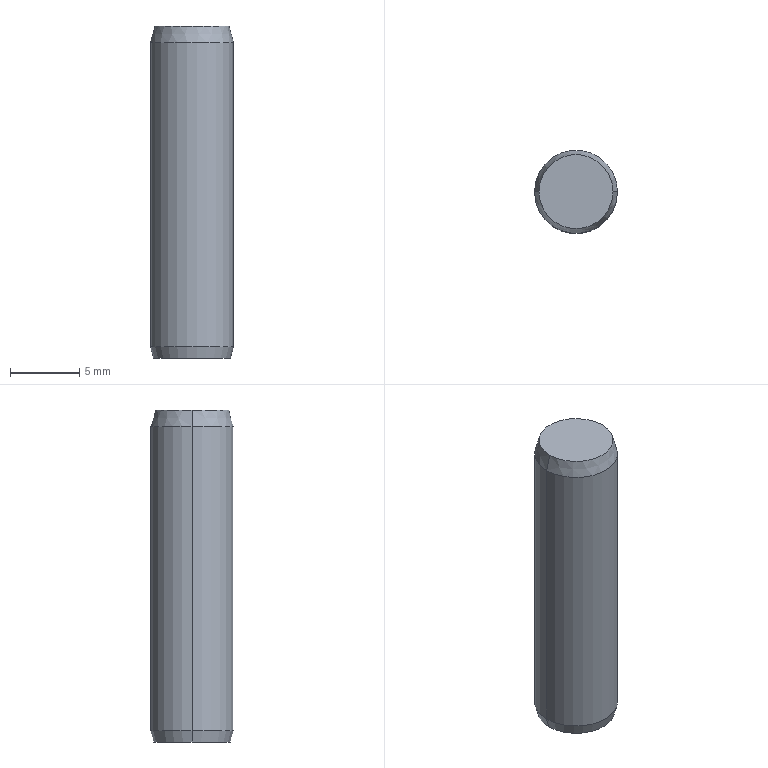Part | SolidWorks | features Chamfer 3, Cut 2, Extrusion 1, RevCut 1 | 1 solid | 16 faces | box 6 x 6 x 24 mm | volume 569.991 mm3 | cone 8 | cylinder 6 | plane 2 | commonest cylinder face diameters 3.464 x2 4.3 x2 6 x2
STEP:
#1=CARTESIAN_POINT('',(1.732,0.,1.418));
#2=VERTEX_POINT('',#1);
#3=CARTESIAN_POINT('',(-1.732,0.,1.418));
#4=VERTEX_POINT('',#3);
#5=CARTESIAN_POINT('',(0.,0.,1.418));
#6=DIRECTION('',(0.,0.,-1.));
#7=DIRECTION('',(-1.,0.,0.));
#8=AXIS2_PLACEMENT_3D('',#5,#6,#7);
#9=CIRCLE('',#8,1.732);
#10=EDGE_CURVE('',#2,#4,#9,.T.);
#11=ORIENTED_EDGE('',*,*,#10,.F.);
#12=CARTESIAN_POINT('',(2.15,0.,1.));
#13=VERTEX_POINT('',#12);
#14=CARTESIAN_POINT('',(2.15,0.,1.));
#15=DIRECTION('',(0.7071,0.,-0.7071));
#16=VECTOR('',#15,1000.);
#17=LINE('',#14,#16);
#18=EDGE_CURVE('',#2,#13,#17,.T.);
#19=ORIENTED_EDGE('',*,*,#18,.T.);
#20=CARTESIAN_POINT('',(-2.15,0.,1.));
#21=VERTEX_POINT('',#20);
#22=CARTESIAN_POINT('',(0.,0.,1.));
#23=DIRECTION('',(0.,0.,-1.));
#24=DIRECTION('',(-1.,0.,0.));
#25=AXIS2_PLACEMENT_3D('',#22,#23,#24);
#26=CIRCLE('',#25,2.15);
#27=EDGE_CURVE('',#13,#21,#26,.T.);
#28=ORIENTED_EDGE('',*,*,#27,.T.);
#29=CARTESIAN_POINT('',(-2.15,0.,1.));
#30=DIRECTION('',(-0.7071,0.,-0.7071));
#31=VECTOR('',#30,1000.);
#32=LINE('',#29,#31);
#33=EDGE_CURVE('',#4,#21,#32,.T.);
#34=ORIENTED_EDGE('',*,*,#33,.F.);
#35=EDGE_LOOP('',(#11,#19,#28,#34));
#36=FACE_OUTER_BOUND('',#35,.T.);
#37=CARTESIAN_POINT('',(0.,0.,1.));
#38=DIRECTION('',(0.,0.,-1.));
#39=DIRECTION('',(-1.,0.,0.));
#40=AXIS2_PLACEMENT_3D('',#37,#38,#39);
#41=CONICAL_SURFACE('',#40,2.15,0.7854);
#42=ADVANCED_FACE('',(#36),#41,.F.);
#43=CARTESIAN_POINT('',(-1.732,0.,10.));
#44=VERTEX_POINT('',#43);
#45=CARTESIAN_POINT('',(1.732,0.,10.));
#46=VERTEX_POINT('',#45);
#47=CARTESIAN_POINT('',(0.,0.,10.));
#48=DIRECTION('',(0.,0.,1.));
#49=DIRECTION('',(1.,0.,0.));
#50=AXIS2_PLACEMENT_3D('',#47,#48,#49);
#51=CIRCLE('',#50,1.732);
#52=EDGE_CURVE('',#44,#46,#51,.T.);
#53=ORIENTED_EDGE('',*,*,#52,.T.);
#54=CARTESIAN_POINT('',(1.732,0.,10.));
#55=DIRECTION('',(0.,0.,-1.));
#56=VECTOR('',#55,1000.);
#57=LINE('',#54,#56);
#58=EDGE_CURVE('',#46,#2,#57,.T.);
#59=ORIENTED_EDGE('',*,*,#58,.T.);
#60=ORIENTED_EDGE('',*,*,#10,.T.);
#61=CARTESIAN_POINT('',(-1.732,0.,10.));
#62=DIRECTION('',(0.,0.,-1.));
#63=VECTOR('',#62,1000.);
#64=LINE('',#61,#63);
#65=EDGE_CURVE('',#44,#4,#64,.T.);
#66=ORIENTED_EDGE('',*,*,#65,.F.);
#67=EDGE_LOOP('',(#53,#59,#60,#66));
#68=FACE_OUTER_BOUND('',#67,.T.);
#69=CARTESIAN_POINT('',(0.,0.,10.));
#70=DIRECTION('',(0.,0.,-1.));
#71=DIRECTION('',(-1.,0.,0.));
#72=AXIS2_PLACEMENT_3D('',#69,#70,#71);
#73=CYLINDRICAL_SURFACE('',#72,1.732);
#74=ADVANCED_FACE('',(#68),#73,.F.);
#75=CARTESIAN_POINT('',(0.,0.,11.));
#76=VERTEX_POINT('',#75);
#77=CARTESIAN_POINT('',(-1.732,0.,10.));
#78=DIRECTION('',(-0.866,0.,-0.5));
#79=VECTOR('',#78,1000.);
#80=LINE('',#77,#79);
#81=EDGE_CURVE('',#76,#44,#80,.T.);
#82=ORIENTED_EDGE('',*,*,#81,.F.);
#83=CARTESIAN_POINT('',(1.732,0.,10.));
#84=DIRECTION('',(0.866,0.,-0.5));
#85=VECTOR('',#84,1000.);
#86=LINE('',#83,#85);
#87=EDGE_CURVE('',#76,#46,#86,.T.);
#88=ORIENTED_EDGE('',*,*,#87,.T.);
#89=ORIENTED_EDGE('',*,*,#52,.F.);
#90=EDGE_LOOP('',(#82,#88,#89));
#91=FACE_OUTER_BOUND('',#90,.T.);
#92=CARTESIAN_POINT('',(0.,0.,10.));
#93=DIRECTION('',(0.,0.,-1.));
#94=DIRECTION('',(-1.,0.,0.));
#95=AXIS2_PLACEMENT_3D('',#92,#93,#94);
#96=CONICAL_SURFACE('',#95,1.732,1.047);
#97=ADVANCED_FACE('',(#91),#96,.F.);
#98=ORIENTED_EDGE('',*,*,#27,.F.);
#99=CARTESIAN_POINT('',(2.15,0.,0.));
#100=VERTEX_POINT('',#99);
#101=CARTESIAN_POINT('',(2.15,0.,1.));
#102=DIRECTION('',(0.,0.,-1.));
#103=VECTOR('',#102,1000.);
#104=LINE('',#101,#103);
#105=EDGE_CURVE('',#13,#100,#104,.T.);
#106=ORIENTED_EDGE('',*,*,#105,.T.);
#107=CARTESIAN_POINT('',(-2.15,0.,0.));
#108=VERTEX_POINT('',#107);
#109=CARTESIAN_POINT('',(0.,0.,0.));
#110=DIRECTION('',(0.,0.,-1.));
#111=DIRECTION('',(-1.,0.,0.));
#112=AXIS2_PLACEMENT_3D('',#109,#110,#111);
#113=CIRCLE('',#112,2.15);
#114=EDGE_CURVE('',#100,#108,#113,.T.);
#115=ORIENTED_EDGE('',*,*,#114,.T.);
#116=CARTESIAN_POINT('',(-2.15,0.,1.));
#117=DIRECTION('',(0.,0.,-1.));
#118=VECTOR('',#117,1000.);
#119=LINE('',#116,#118);
#120=EDGE_CURVE('',#21,#108,#119,.T.);
#121=ORIENTED_EDGE('',*,*,#120,.F.);
#122=EDGE_LOOP('',(#98,#106,#115,#121));
#123=FACE_OUTER_BOUND('',#122,.T.);
#124=CARTESIAN_POINT('',(0.,0.,1.));
#125=DIRECTION('',(0.,0.,-1.));
#126=DIRECTION('',(-1.,0.,0.));
#127=AXIS2_PLACEMENT_3D('',#124,#125,#126);
#128=CYLINDRICAL_SURFACE('',#127,2.15);
#129=ADVANCED_FACE('',(#123),#128,.F.);
#130=CARTESIAN_POINT('',(-2.786,0.,0.));
#131=VERTEX_POINT('',#130);
#132=CARTESIAN_POINT('',(2.786,0.,0.));
#133=VERTEX_POINT('',#132);
#134=CARTESIAN_POINT('',(0.,0.,0.));
#135=DIRECTION('',(0.,0.,-1.));
#136=DIRECTION('',(1.,0.,0.));
#137=AXIS2_PLACEMENT_3D('',#134,#135,#136);
#138=CIRCLE('',#137,2.786);
#139=EDGE_CURVE('',#131,#133,#138,.T.);
#140=ORIENTED_EDGE('',*,*,#139,.F.);
#141=CARTESIAN_POINT('',(-3.,0.,0.8));
#142=VERTEX_POINT('',#141);
#143=CARTESIAN_POINT('',(-3.,0.,0.8));
#144=DIRECTION('',(-0.2588,0.,0.9659));
#145=VECTOR('',#144,1000.);
#146=LINE('',#143,#145);
#147=EDGE_CURVE('',#131,#142,#146,.T.);
#148=ORIENTED_EDGE('',*,*,#147,.T.);
#149=CARTESIAN_POINT('',(3.,0.,0.8));
#150=VERTEX_POINT('',#149);
#151=CARTESIAN_POINT('',(0.,0.,0.8));
#152=DIRECTION('',(0.,0.,1.));
#153=DIRECTION('',(1.,0.,0.));
#154=AXIS2_PLACEMENT_3D('',#151,#152,#153);
#155=CIRCLE('',#154,3.);
#156=EDGE_CURVE('',#150,#142,#155,.T.);
#157=ORIENTED_EDGE('',*,*,#156,.F.);
#158=CARTESIAN_POINT('',(3.,0.,0.8));
#159=DIRECTION('',(0.2588,0.,0.9659));
#160=VECTOR('',#159,1000.);
#161=LINE('',#158,#160);
#162=EDGE_CURVE('',#133,#150,#161,.T.);
#163=ORIENTED_EDGE('',*,*,#162,.F.);
#164=EDGE_LOOP('',(#140,#148,#157,#163));
#165=FACE_OUTER_BOUND('',#164,.T.);
#166=CARTESIAN_POINT('',(0.,0.,0.8));
#167=DIRECTION('',(0.,0.,1.));
#168=DIRECTION('',(1.,0.,0.));
#169=AXIS2_PLACEMENT_3D('',#166,#167,#168);
#170=CONICAL_SURFACE('',#169,3.,0.2618);
#171=ADVANCED_FACE('',(#165),#170,.T.);
#172=CARTESIAN_POINT('',(2.678,0.,24.));
#173=VERTEX_POINT('',#172);
#174=CARTESIAN_POINT('',(-2.678,0.,24.));
#175=VERTEX_POINT('',#174);
#176=CARTESIAN_POINT('',(0.,0.,24.));
#177=DIRECTION('',(0.,0.,1.));
#178=DIRECTION('',(1.,0.,0.));
#179=AXIS2_PLACEMENT_3D('',#176,#177,#178);
#180=CIRCLE('',#179,2.678);
#181=EDGE_CURVE('',#173,#175,#180,.T.);
#182=ORIENTED_EDGE('',*,*,#181,.F.);
#183=CARTESIAN_POINT('',(3.,0.,22.8));
#184=VERTEX_POINT('',#183);
#185=CARTESIAN_POINT('',(2.678,0.,24.));
#186=DIRECTION('',(0.2588,0.,-0.9659));
#187=VECTOR('',#186,1000.);
#188=LINE('',#185,#187);
#189=EDGE_CURVE('',#173,#184,#188,.T.);
#190=ORIENTED_EDGE('',*,*,#189,.T.);
#191=CARTESIAN_POINT('',(-3.,0.,22.8));
#192=VERTEX_POINT('',#191);
#193=CARTESIAN_POINT('',(0.,0.,22.8));
#194=DIRECTION('',(0.,0.,-1.));
#195=DIRECTION('',(1.,0.,0.));
#196=AXIS2_PLACEMENT_3D('',#193,#194,#195);
#197=CIRCLE('',#196,3.);
#198=EDGE_CURVE('',#192,#184,#197,.T.);
#199=ORIENTED_EDGE('',*,*,#198,.F.);
#200=CARTESIAN_POINT('',(-2.678,0.,24.));
#201=DIRECTION('',(-0.2588,0.,-0.9659));
#202=VECTOR('',#201,1000.);
#203=LINE('',#200,#202);
#204=EDGE_CURVE('',#175,#192,#203,.T.);
#205=ORIENTED_EDGE('',*,*,#204,.F.);
#206=EDGE_LOOP('',(#182,#190,#199,#205));
#207=FACE_OUTER_BOUND('',#206,.T.);
#208=CARTESIAN_POINT('',(0.,0.,24.));
#209=DIRECTION('',(0.,0.,-1.));
#210=DIRECTION('',(-1.,0.,0.));
#211=AXIS2_PLACEMENT_3D('',#208,#209,#210);
#212=CONICAL_SURFACE('',#211,2.678,0.2618);
#213=ADVANCED_FACE('',(#207),#212,.T.);
#214=ORIENTED_EDGE('',*,*,#198,.T.);
#215=CARTESIAN_POINT('',(3.,0.,24.));
#216=DIRECTION('',(0.,0.,-1.));
#217=VECTOR('',#216,1000.);
#218=LINE('',#215,#217);
#219=EDGE_CURVE('',#184,#150,#218,.T.);
#220=ORIENTED_EDGE('',*,*,#219,.T.);
#221=ORIENTED_EDGE('',*,*,#156,.T.);
#222=CARTESIAN_POINT('',(-3.,0.,24.));
#223=DIRECTION('',(0.,0.,-1.));
#224=VECTOR('',#223,1000.);
#225=LINE('',#222,#224);
#226=EDGE_CURVE('',#192,#142,#225,.T.);
#227=ORIENTED_EDGE('',*,*,#226,.F.);
#228=EDGE_LOOP('',(#214,#220,#221,#227));
#229=FACE_OUTER_BOUND('',#228,.T.);
#230=CARTESIAN_POINT('',(0.,0.,24.));
#231=DIRECTION('',(0.,0.,-1.));
#232=DIRECTION('',(-1.,0.,0.));
#233=AXIS2_PLACEMENT_3D('',#230,#231,#232);
#234=CYLINDRICAL_SURFACE('',#233,3.);
#235=ADVANCED_FACE('',(#229),#234,.T.);
#236=ORIENTED_EDGE('',*,*,#219,.F.);
#237=CARTESIAN_POINT('',(0.,0.,22.8));
#238=DIRECTION('',(0.,0.,-1.));
#239=DIRECTION('',(1.,0.,0.));
#240=AXIS2_PLACEMENT_3D('',#237,#238,#239);
#241=CIRCLE('',#240,3.);
#242=EDGE_CURVE('',#184,#192,#241,.T.);
#243=ORIENTED_EDGE('',*,*,#242,.T.);
#244=ORIENTED_EDGE('',*,*,#226,.T.);
#245=CARTESIAN_POINT('',(0.,0.,0.8));
#246=DIRECTION('',(0.,0.,1.));
#247=DIRECTION('',(1.,0.,0.));
#248=AXIS2_PLACEMENT_3D('',#245,#246,#247);
#249=CIRCLE('',#248,3.);
#250=EDGE_CURVE('',#142,#150,#249,.T.);
#251=ORIENTED_EDGE('',*,*,#250,.T.);
#252=EDGE_LOOP('',(#236,#243,#244,#251));
#253=FACE_OUTER_BOUND('',#252,.T.);
#254=CARTESIAN_POINT('',(0.,0.,24.));
#255=DIRECTION('',(0.,0.,-1.));
#256=DIRECTION('',(-1.,0.,0.));
#257=AXIS2_PLACEMENT_3D('',#254,#255,#256);
#258=CYLINDRICAL_SURFACE('',#257,3.);
#259=ADVANCED_FACE('',(#253),#258,.T.);
#260=CARTESIAN_POINT('',(0.,0.,24.));
#261=DIRECTION('',(0.,0.,1.));
#262=DIRECTION('',(1.,0.,0.));
#263=AXIS2_PLACEMENT_3D('',#260,#261,#262);
#264=CIRCLE('',#263,2.678);
#265=EDGE_CURVE('',#175,#173,#264,.T.);
#266=ORIENTED_EDGE('',*,*,#265,.T.);
#267=ORIENTED_EDGE('',*,*,#181,.T.);
#268=EDGE_LOOP('',(#266,#267));
#269=FACE_OUTER_BOUND('',#268,.T.);
#270=CARTESIAN_POINT('',(0.,0.,24.));
#271=DIRECTION('',(0.,0.,1.));
#272=DIRECTION('',(1.,0.,0.));
#273=AXIS2_PLACEMENT_3D('',#270,#271,#272);
#274=PLANE('',#273);
#275=ADVANCED_FACE('',(#269),#274,.T.);
#276=CARTESIAN_POINT('',(0.,0.,0.));
#277=DIRECTION('',(0.,0.,-1.));
#278=DIRECTION('',(-1.,0.,0.));
#279=AXIS2_PLACEMENT_3D('',#276,#277,#278);
#280=CIRCLE('',#279,2.15);
#281=EDGE_CURVE('',#108,#100,#280,.T.);
#282=ORIENTED_EDGE('',*,*,#281,.F.);
#283=ORIENTED_EDGE('',*,*,#114,.F.);
#284=EDGE_LOOP('',(#282,#283));
#285=FACE_BOUND('',#284,.T.);
#286=CARTESIAN_POINT('',(0.,0.,0.));
#287=DIRECTION('',(0.,0.,-1.));
#288=DIRECTION('',(1.,0.,0.));
#289=AXIS2_PLACEMENT_3D('',#286,#287,#288);
#290=CIRCLE('',#289,2.786);
#291=EDGE_CURVE('',#133,#131,#290,.T.);
#292=ORIENTED_EDGE('',*,*,#291,.T.);
#293=ORIENTED_EDGE('',*,*,#139,.T.);
#294=EDGE_LOOP('',(#292,#293));
#295=FACE_OUTER_BOUND('',#294,.T.);
#296=CARTESIAN_POINT('',(0.,0.,0.));
#297=DIRECTION('',(0.,0.,1.));
#298=DIRECTION('',(1.,0.,0.));
#299=AXIS2_PLACEMENT_3D('',#296,#297,#298);
#300=PLANE('',#299);
#301=ADVANCED_FACE('',(#285,#295),#300,.F.);
#302=ORIENTED_EDGE('',*,*,#189,.F.);
#303=ORIENTED_EDGE('',*,*,#265,.F.);
#304=ORIENTED_EDGE('',*,*,#204,.T.);
#305=ORIENTED_EDGE('',*,*,#242,.F.);
#306=EDGE_LOOP('',(#302,#303,#304,#305));
#307=FACE_OUTER_BOUND('',#306,.T.);
#308=CARTESIAN_POINT('',(0.,0.,24.));
#309=DIRECTION('',(0.,0.,-1.));
#310=DIRECTION('',(-1.,0.,0.));
#311=AXIS2_PLACEMENT_3D('',#308,#309,#310);
#312=CONICAL_SURFACE('',#311,2.678,0.2618);
#313=ADVANCED_FACE('',(#307),#312,.T.);
#314=ORIENTED_EDGE('',*,*,#147,.F.);
#315=ORIENTED_EDGE('',*,*,#291,.F.);
#316=ORIENTED_EDGE('',*,*,#162,.T.);
#317=ORIENTED_EDGE('',*,*,#250,.F.);
#318=EDGE_LOOP('',(#314,#315,#316,#317));
#319=FACE_OUTER_BOUND('',#318,.T.);
#320=CARTESIAN_POINT('',(0.,0.,0.8));
#321=DIRECTION('',(0.,0.,1.));
#322=DIRECTION('',(1.,0.,0.));
#323=AXIS2_PLACEMENT_3D('',#320,#321,#322);
#324=CONICAL_SURFACE('',#323,3.,0.2618);
#325=ADVANCED_FACE('',(#319),#324,.T.);
#326=ORIENTED_EDGE('',*,*,#105,.F.);
#327=CARTESIAN_POINT('',(0.,0.,1.));
#328=DIRECTION('',(0.,0.,-1.));
#329=DIRECTION('',(-1.,0.,0.));
#330=AXIS2_PLACEMENT_3D('',#327,#328,#329);
#331=CIRCLE('',#330,2.15);
#332=EDGE_CURVE('',#21,#13,#331,.T.);
#333=ORIENTED_EDGE('',*,*,#332,.F.);
#334=ORIENTED_EDGE('',*,*,#120,.T.);
#335=ORIENTED_EDGE('',*,*,#281,.T.);
#336=EDGE_LOOP('',(#326,#333,#334,#335));
#337=FACE_OUTER_BOUND('',#336,.T.);
#338=CARTESIAN_POINT('',(0.,0.,1.));
#339=DIRECTION('',(0.,0.,-1.));
#340=DIRECTION('',(-1.,0.,0.));
#341=AXIS2_PLACEMENT_3D('',#338,#339,#340);
#342=CYLINDRICAL_SURFACE('',#341,2.15);
#343=ADVANCED_FACE('',(#337),#342,.F.);
#344=ORIENTED_EDGE('',*,*,#87,.F.);
#345=ORIENTED_EDGE('',*,*,#81,.T.);
#346=CARTESIAN_POINT('',(0.,0.,10.));
#347=DIRECTION('',(0.,0.,1.));
#348=DIRECTION('',(1.,0.,0.));
#349=AXIS2_PLACEMENT_3D('',#346,#347,#348);
#350=CIRCLE('',#349,1.732);
#351=EDGE_CURVE('',#46,#44,#350,.T.);
#352=ORIENTED_EDGE('',*,*,#351,.F.);
#353=EDGE_LOOP('',(#344,#345,#352));
#354=FACE_OUTER_BOUND('',#353,.T.);
#355=CARTESIAN_POINT('',(0.,0.,10.));
#356=DIRECTION('',(0.,0.,-1.));
#357=DIRECTION('',(-1.,0.,0.));
#358=AXIS2_PLACEMENT_3D('',#355,#356,#357);
#359=CONICAL_SURFACE('',#358,1.732,1.047);
#360=ADVANCED_FACE('',(#354),#359,.F.);
#361=ORIENTED_EDGE('',*,*,#58,.F.);
#362=ORIENTED_EDGE('',*,*,#351,.T.);
#363=ORIENTED_EDGE('',*,*,#65,.T.);
#364=CARTESIAN_POINT('',(0.,0.,1.418));
#365=DIRECTION('',(0.,0.,-1.));
#366=DIRECTION('',(-1.,0.,0.));
#367=AXIS2_PLACEMENT_3D('',#364,#365,#366);
#368=CIRCLE('',#367,1.732);
#369=EDGE_CURVE('',#4,#2,#368,.T.);
#370=ORIENTED_EDGE('',*,*,#369,.T.);
#371=EDGE_LOOP('',(#361,#362,#363,#370));
#372=FACE_OUTER_BOUND('',#371,.T.);
#373=CARTESIAN_POINT('',(0.,0.,10.));
#374=DIRECTION('',(0.,0.,-1.));
#375=DIRECTION('',(-1.,0.,0.));
#376=AXIS2_PLACEMENT_3D('',#373,#374,#375);
#377=CYLINDRICAL_SURFACE('',#376,1.732);
#378=ADVANCED_FACE('',(#372),#377,.F.);
#379=ORIENTED_EDGE('',*,*,#18,.F.);
#380=ORIENTED_EDGE('',*,*,#369,.F.);
#381=ORIENTED_EDGE('',*,*,#33,.T.);
#382=ORIENTED_EDGE('',*,*,#332,.T.);
#383=EDGE_LOOP('',(#379,#380,#381,#382));
#384=FACE_OUTER_BOUND('',#383,.T.);
#385=CARTESIAN_POINT('',(0.,0.,1.));
#386=DIRECTION('',(0.,0.,-1.));
#387=DIRECTION('',(-1.,0.,0.));
#388=AXIS2_PLACEMENT_3D('',#385,#386,#387);
#389=CONICAL_SURFACE('',#388,2.15,0.7854);
#390=ADVANCED_FACE('',(#384),#389,.F.);
#391=CLOSED_SHELL('',(#42,#74,#97,#129,#171,#213,#235,#259,#275,#301,#313,#325,#343,#360,#378,#390));
#392=MANIFOLD_SOLID_BREP('',#391);
#393=CARTESIAN_POINT('',(0.,0.,0.));
#394=DIRECTION('',(0.,0.,1.));
#395=DIRECTION('',(1.,0.,0.));
#396=AXIS2_PLACEMENT_3D('',#393,#394,#395);
#397=(LENGTH_UNIT()NAMED_UNIT(*)SI_UNIT(.MILLI.,.METRE.));
#398=UNCERTAINTY_MEASURE_WITH_UNIT(LENGTH_MEASURE(0.00001),#397,'','');
#399=(NAMED_UNIT(*)PLANE_ANGLE_UNIT()SI_UNIT($,.RADIAN.));
#400=(NAMED_UNIT(*)SI_UNIT($,.STERADIAN.)SOLID_ANGLE_UNIT());
#401=(GEOMETRIC_REPRESENTATION_CONTEXT(3)GLOBAL_UNCERTAINTY_ASSIGNED_CONTEXT((#398))GLOBAL_UNIT_ASSIGNED_CONTEXT((#397,#399,#400))REPRESENTATION_CONTEXT('',''));
#402=ADVANCED_BREP_SHAPE_REPRESENTATION('',(#392,#396),#401);